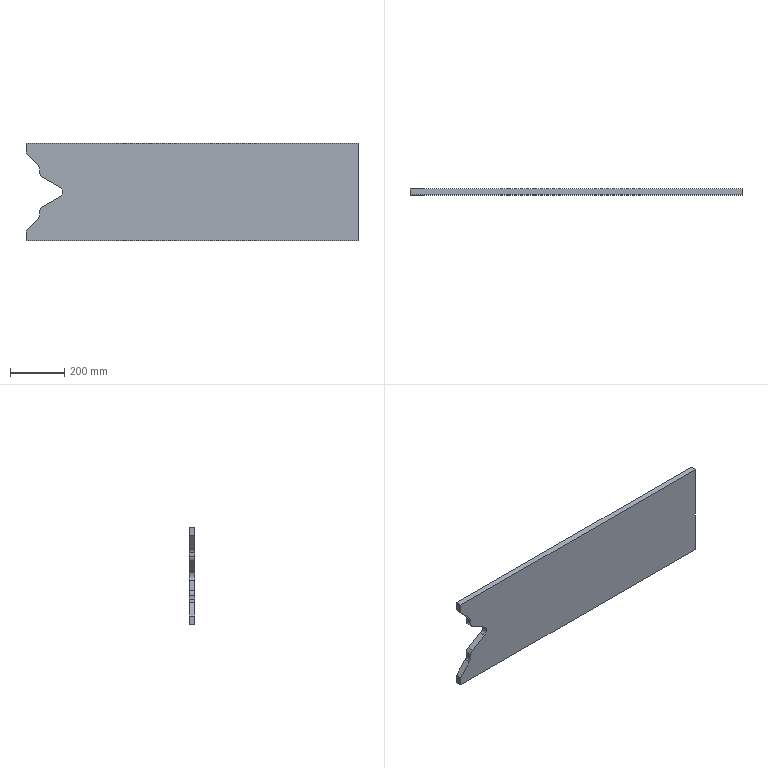Part | NX | features 底座(默认<按焊接>) 2 | 1 solid | 18 faces | box 1222 x 21.82 x 360 mm | volume 9202426 mm3 | plane 13 | cylinder 5 | commonest cylinder face diameters 40 x4 42 x1
STEP:
#1=CARTESIAN_POINT('',(2311.685,545.5,-58.7));
#2=VERTEX_POINT('',#1);
#3=CARTESIAN_POINT('',(2311.685,567.32,-58.7));
#4=VERTEX_POINT('',#3);
#5=CARTESIAN_POINT('',(2311.685,567.32,-58.7));
#6=DIRECTION('',(0.,1.,0.));
#7=VECTOR('',#6,1000.);
#8=LINE('',#5,#7);
#9=EDGE_CURVE('',#2,#4,#8,.T.);
#10=ORIENTED_EDGE('',*,*,#9,.F.);
#11=CARTESIAN_POINT('',(2311.685,545.5,-26.));
#12=VERTEX_POINT('',#11);
#13=CARTESIAN_POINT('',(2311.685,545.5,-386.));
#14=DIRECTION('',(0.,0.,1.));
#15=VECTOR('',#14,1000.);
#16=LINE('',#13,#15);
#17=EDGE_CURVE('',#2,#12,#16,.T.);
#18=ORIENTED_EDGE('',*,*,#17,.T.);
#19=CARTESIAN_POINT('',(2311.685,567.32,-26.));
#20=VERTEX_POINT('',#19);
#21=CARTESIAN_POINT('',(2311.685,567.32,-26.));
#22=DIRECTION('',(0.,-1.,0.));
#23=VECTOR('',#22,1000.);
#24=LINE('',#21,#23);
#25=EDGE_CURVE('',#20,#12,#24,.T.);
#26=ORIENTED_EDGE('',*,*,#25,.F.);
#27=CARTESIAN_POINT('',(2311.685,567.32,-386.));
#28=DIRECTION('',(0.,0.,1.));
#29=VECTOR('',#28,1000.);
#30=LINE('',#27,#29);
#31=EDGE_CURVE('',#4,#20,#30,.T.);
#32=ORIENTED_EDGE('',*,*,#31,.F.);
#33=EDGE_LOOP('',(#10,#18,#26,#32));
#34=FACE_BOUND('',#33,.T.);
#35=CARTESIAN_POINT('',(2311.685,567.32,-386.));
#36=DIRECTION('',(-1.,0.,0.));
#37=DIRECTION('',(0.,0.,1.));
#38=AXIS2_PLACEMENT_3D('',#35,#36,#37);
#39=PLANE('',#38);
#40=ADVANCED_FACE('',(#34),#39,.T.);
#41=CARTESIAN_POINT('',(3533.685,567.32,-26.));
#42=VERTEX_POINT('',#41);
#43=CARTESIAN_POINT('',(3533.685,545.5,-26.));
#44=VERTEX_POINT('',#43);
#45=CARTESIAN_POINT('',(3533.685,567.32,-26.));
#46=DIRECTION('',(0.,-1.,0.));
#47=VECTOR('',#46,1000.);
#48=LINE('',#45,#47);
#49=EDGE_CURVE('',#42,#44,#48,.T.);
#50=ORIENTED_EDGE('',*,*,#49,.F.);
#51=CARTESIAN_POINT('',(3533.685,567.32,-26.));
#52=DIRECTION('',(-1.,0.,0.));
#53=VECTOR('',#52,1000.);
#54=LINE('',#51,#53);
#55=EDGE_CURVE('',#42,#20,#54,.T.);
#56=ORIENTED_EDGE('',*,*,#55,.T.);
#57=ORIENTED_EDGE('',*,*,#25,.T.);
#58=CARTESIAN_POINT('',(3533.685,545.5,-26.));
#59=DIRECTION('',(-1.,0.,0.));
#60=VECTOR('',#59,1000.);
#61=LINE('',#58,#60);
#62=EDGE_CURVE('',#44,#12,#61,.T.);
#63=ORIENTED_EDGE('',*,*,#62,.F.);
#64=EDGE_LOOP('',(#50,#56,#57,#63));
#65=FACE_BOUND('',#64,.T.);
#66=CARTESIAN_POINT('',(3533.685,545.5,-26.));
#67=DIRECTION('',(0.,0.,-1.));
#68=DIRECTION('',(-1.,0.,0.));
#69=AXIS2_PLACEMENT_3D('',#66,#67,#68);
#70=PLANE('',#69);
#71=ADVANCED_FACE('',(#65),#70,.F.);
#72=CARTESIAN_POINT('',(3533.685,567.32,-386.));
#73=VERTEX_POINT('',#72);
#74=CARTESIAN_POINT('',(3533.685,545.5,-386.));
#75=VERTEX_POINT('',#74);
#76=CARTESIAN_POINT('',(3533.685,567.32,-386.));
#77=DIRECTION('',(0.,-1.,0.));
#78=VECTOR('',#77,1000.);
#79=LINE('',#76,#78);
#80=EDGE_CURVE('',#73,#75,#79,.T.);
#81=ORIENTED_EDGE('',*,*,#80,.T.);
#82=CARTESIAN_POINT('',(2311.685,545.5,-386.));
#83=VERTEX_POINT('',#82);
#84=CARTESIAN_POINT('',(3533.685,545.5,-386.));
#85=DIRECTION('',(-1.,0.,0.));
#86=VECTOR('',#85,1000.);
#87=LINE('',#84,#86);
#88=EDGE_CURVE('',#75,#83,#87,.T.);
#89=ORIENTED_EDGE('',*,*,#88,.T.);
#90=CARTESIAN_POINT('',(2311.685,567.32,-386.));
#91=VERTEX_POINT('',#90);
#92=CARTESIAN_POINT('',(2311.685,567.32,-386.));
#93=DIRECTION('',(0.,-1.,0.));
#94=VECTOR('',#93,1000.);
#95=LINE('',#92,#94);
#96=EDGE_CURVE('',#91,#83,#95,.T.);
#97=ORIENTED_EDGE('',*,*,#96,.F.);
#98=CARTESIAN_POINT('',(3533.685,567.32,-386.));
#99=DIRECTION('',(-1.,0.,0.));
#100=VECTOR('',#99,1000.);
#101=LINE('',#98,#100);
#102=EDGE_CURVE('',#73,#91,#101,.T.);
#103=ORIENTED_EDGE('',*,*,#102,.F.);
#104=EDGE_LOOP('',(#81,#89,#97,#103));
#105=FACE_BOUND('',#104,.T.);
#106=CARTESIAN_POINT('',(3533.685,545.5,-386.));
#107=DIRECTION('',(0.,0.,-1.));
#108=DIRECTION('',(-1.,0.,0.));
#109=AXIS2_PLACEMENT_3D('',#106,#107,#108);
#110=PLANE('',#109);
#111=ADVANCED_FACE('',(#105),#110,.T.);
#112=CARTESIAN_POINT('',(2311.685,567.32,-353.3));
#113=VERTEX_POINT('',#112);
#114=CARTESIAN_POINT('',(2311.685,545.5,-353.3));
#115=VERTEX_POINT('',#114);
#116=CARTESIAN_POINT('',(2311.685,567.32,-353.3));
#117=DIRECTION('',(0.,-1.,0.));
#118=VECTOR('',#117,1000.);
#119=LINE('',#116,#118);
#120=EDGE_CURVE('',#113,#115,#119,.T.);
#121=ORIENTED_EDGE('',*,*,#120,.F.);
#122=CARTESIAN_POINT('',(2311.685,567.32,-386.));
#123=DIRECTION('',(0.,0.,1.));
#124=VECTOR('',#123,1000.);
#125=LINE('',#122,#124);
#126=EDGE_CURVE('',#91,#113,#125,.T.);
#127=ORIENTED_EDGE('',*,*,#126,.F.);
#128=ORIENTED_EDGE('',*,*,#96,.T.);
#129=CARTESIAN_POINT('',(2311.685,545.5,-386.));
#130=DIRECTION('',(0.,0.,1.));
#131=VECTOR('',#130,1000.);
#132=LINE('',#129,#131);
#133=EDGE_CURVE('',#83,#115,#132,.T.);
#134=ORIENTED_EDGE('',*,*,#133,.T.);
#135=EDGE_LOOP('',(#121,#127,#128,#134));
#136=FACE_BOUND('',#135,.T.);
#137=CARTESIAN_POINT('',(2311.685,567.32,-386.));
#138=DIRECTION('',(-1.,0.,0.));
#139=DIRECTION('',(0.,0.,1.));
#140=AXIS2_PLACEMENT_3D('',#137,#138,#139);
#141=PLANE('',#140);
#142=ADVANCED_FACE('',(#136),#141,.T.);
#143=ORIENTED_EDGE('',*,*,#17,.F.);
#144=CARTESIAN_POINT('',(2356.433,545.5,-107.546));
#145=VERTEX_POINT('',#144);
#146=CARTESIAN_POINT('',(2311.685,545.5,-58.7));
#147=DIRECTION('',(-0.6755,0.,0.7374));
#148=VECTOR('',#147,1000.);
#149=LINE('',#146,#148);
#150=EDGE_CURVE('',#145,#2,#149,.T.);
#151=ORIENTED_EDGE('',*,*,#150,.F.);
#152=CARTESIAN_POINT('',(2361.685,545.5,-121.056));
#153=VERTEX_POINT('',#152);
#154=CARTESIAN_POINT('',(2341.685,545.5,-121.056));
#155=DIRECTION('',(0.,-1.,0.));
#156=DIRECTION('',(0.,0.,-1.));
#157=AXIS2_PLACEMENT_3D('',#154,#155,#156);
#158=CIRCLE('',#157,20.);
#159=EDGE_CURVE('',#153,#145,#158,.T.);
#160=ORIENTED_EDGE('',*,*,#159,.F.);
#161=CARTESIAN_POINT('',(2361.685,545.5,-133.717));
#162=VERTEX_POINT('',#161);
#163=CARTESIAN_POINT('',(2361.685,545.5,-121.056));
#164=DIRECTION('',(0.,0.,1.));
#165=VECTOR('',#164,1000.);
#166=LINE('',#163,#165);
#167=EDGE_CURVE('',#162,#153,#166,.T.);
#168=ORIENTED_EDGE('',*,*,#167,.F.);
#169=CARTESIAN_POINT('',(2372.64,545.5,-151.555));
#170=VERTEX_POINT('',#169);
#171=CARTESIAN_POINT('',(2381.685,545.5,-133.717));
#172=DIRECTION('',(0.,1.,0.));
#173=DIRECTION('',(0.,0.,1.));
#174=AXIS2_PLACEMENT_3D('',#171,#172,#173);
#175=CIRCLE('',#174,20.);
#176=EDGE_CURVE('',#170,#162,#175,.T.);
#177=ORIENTED_EDGE('',*,*,#176,.F.);
#178=CARTESIAN_POINT('',(2436.093,545.5,-187.76));
#179=VERTEX_POINT('',#178);
#180=CARTESIAN_POINT('',(2372.64,545.5,-151.555));
#181=DIRECTION('',(-0.8686,0.,0.4956));
#182=VECTOR('',#181,1000.);
#183=LINE('',#180,#182);
#184=EDGE_CURVE('',#179,#170,#183,.T.);
#185=ORIENTED_EDGE('',*,*,#184,.F.);
#186=CARTESIAN_POINT('',(2436.093,545.5,-224.24));
#187=VERTEX_POINT('',#186);
#188=CARTESIAN_POINT('',(2425.685,545.5,-206.));
#189=DIRECTION('',(0.,-1.,0.));
#190=DIRECTION('',(0.,0.,-1.));
#191=AXIS2_PLACEMENT_3D('',#188,#189,#190);
#192=CIRCLE('',#191,21.);
#193=EDGE_CURVE('',#187,#179,#192,.T.);
#194=ORIENTED_EDGE('',*,*,#193,.F.);
#195=CARTESIAN_POINT('',(2372.64,545.5,-260.445));
#196=VERTEX_POINT('',#195);
#197=CARTESIAN_POINT('',(2372.64,545.5,-260.445));
#198=DIRECTION('',(0.8686,0.,0.4956));
#199=VECTOR('',#198,1000.);
#200=LINE('',#197,#199);
#201=EDGE_CURVE('',#196,#187,#200,.T.);
#202=ORIENTED_EDGE('',*,*,#201,.F.);
#203=CARTESIAN_POINT('',(2361.685,545.5,-278.283));
#204=VERTEX_POINT('',#203);
#205=CARTESIAN_POINT('',(2381.685,545.5,-278.283));
#206=DIRECTION('',(0.,1.,0.));
#207=DIRECTION('',(0.,0.,-1.));
#208=AXIS2_PLACEMENT_3D('',#205,#206,#207);
#209=CIRCLE('',#208,20.);
#210=EDGE_CURVE('',#204,#196,#209,.T.);
#211=ORIENTED_EDGE('',*,*,#210,.F.);
#212=CARTESIAN_POINT('',(2361.685,545.5,-290.944));
#213=VERTEX_POINT('',#212);
#214=CARTESIAN_POINT('',(2361.685,545.5,-290.944));
#215=DIRECTION('',(0.,0.,1.));
#216=VECTOR('',#215,1000.);
#217=LINE('',#214,#216);
#218=EDGE_CURVE('',#213,#204,#217,.T.);
#219=ORIENTED_EDGE('',*,*,#218,.F.);
#220=CARTESIAN_POINT('',(2356.433,545.5,-304.454));
#221=VERTEX_POINT('',#220);
#222=CARTESIAN_POINT('',(2341.685,545.5,-290.944));
#223=DIRECTION('',(0.,-1.,0.));
#224=DIRECTION('',(0.,0.,1.));
#225=AXIS2_PLACEMENT_3D('',#222,#223,#224);
#226=CIRCLE('',#225,20.);
#227=EDGE_CURVE('',#221,#213,#226,.T.);
#228=ORIENTED_EDGE('',*,*,#227,.F.);
#229=CARTESIAN_POINT('',(2311.685,545.5,-353.3));
#230=DIRECTION('',(0.6755,0.,0.7374));
#231=VECTOR('',#230,1000.);
#232=LINE('',#229,#231);
#233=EDGE_CURVE('',#115,#221,#232,.T.);
#234=ORIENTED_EDGE('',*,*,#233,.F.);
#235=ORIENTED_EDGE('',*,*,#133,.F.);
#236=ORIENTED_EDGE('',*,*,#88,.F.);
#237=CARTESIAN_POINT('',(3533.685,545.5,-386.));
#238=DIRECTION('',(0.,0.,1.));
#239=VECTOR('',#238,1000.);
#240=LINE('',#237,#239);
#241=EDGE_CURVE('',#75,#44,#240,.T.);
#242=ORIENTED_EDGE('',*,*,#241,.T.);
#243=ORIENTED_EDGE('',*,*,#62,.T.);
#244=EDGE_LOOP('',(#143,#151,#160,#168,#177,#185,#194,#202,#211,#219,#228,#234,#235,#236,#242,#243));
#245=FACE_BOUND('',#244,.T.);
#246=CARTESIAN_POINT('',(3533.685,545.5,-386.));
#247=DIRECTION('',(0.,1.,0.));
#248=DIRECTION('',(0.,0.,1.));
#249=AXIS2_PLACEMENT_3D('',#246,#247,#248);
#250=PLANE('',#249);
#251=ADVANCED_FACE('',(#245),#250,.F.);
#252=ORIENTED_EDGE('',*,*,#49,.T.);
#253=ORIENTED_EDGE('',*,*,#241,.F.);
#254=ORIENTED_EDGE('',*,*,#80,.F.);
#255=CARTESIAN_POINT('',(3533.685,567.32,-386.));
#256=DIRECTION('',(0.,0.,1.));
#257=VECTOR('',#256,1000.);
#258=LINE('',#255,#257);
#259=EDGE_CURVE('',#73,#42,#258,.T.);
#260=ORIENTED_EDGE('',*,*,#259,.T.);
#261=EDGE_LOOP('',(#252,#253,#254,#260));
#262=FACE_BOUND('',#261,.T.);
#263=CARTESIAN_POINT('',(3533.685,567.32,-386.));
#264=DIRECTION('',(-1.,0.,0.));
#265=DIRECTION('',(0.,0.,1.));
#266=AXIS2_PLACEMENT_3D('',#263,#264,#265);
#267=PLANE('',#266);
#268=ADVANCED_FACE('',(#262),#267,.F.);
#269=CARTESIAN_POINT('',(2356.433,567.32,-107.546));
#270=VERTEX_POINT('',#269);
#271=CARTESIAN_POINT('',(3032.295,567.32,-845.317));
#272=DIRECTION('',(0.6755,0.,-0.7374));
#273=VECTOR('',#272,1000.);
#274=LINE('',#271,#273);
#275=EDGE_CURVE('',#4,#270,#274,.T.);
#276=ORIENTED_EDGE('',*,*,#275,.F.);
#277=ORIENTED_EDGE('',*,*,#31,.T.);
#278=ORIENTED_EDGE('',*,*,#55,.F.);
#279=ORIENTED_EDGE('',*,*,#259,.F.);
#280=ORIENTED_EDGE('',*,*,#102,.T.);
#281=ORIENTED_EDGE('',*,*,#126,.T.);
#282=CARTESIAN_POINT('',(2356.433,567.32,-304.454));
#283=VERTEX_POINT('',#282);
#284=CARTESIAN_POINT('',(2852.984,567.32,237.581));
#285=DIRECTION('',(-0.6755,0.,-0.7374));
#286=VECTOR('',#285,1000.);
#287=LINE('',#284,#286);
#288=EDGE_CURVE('',#283,#113,#287,.T.);
#289=ORIENTED_EDGE('',*,*,#288,.F.);
#290=CARTESIAN_POINT('',(2361.685,567.32,-290.944));
#291=VERTEX_POINT('',#290);
#292=CARTESIAN_POINT('',(2341.685,567.32,-290.944));
#293=DIRECTION('',(0.,1.,0.));
#294=DIRECTION('',(0.,0.,1.));
#295=AXIS2_PLACEMENT_3D('',#292,#293,#294);
#296=CIRCLE('',#295,20.);
#297=EDGE_CURVE('',#291,#283,#296,.T.);
#298=ORIENTED_EDGE('',*,*,#297,.F.);
#299=CARTESIAN_POINT('',(2361.685,567.32,-278.283));
#300=VERTEX_POINT('',#299);
#301=CARTESIAN_POINT('',(2361.685,567.32,-386.));
#302=DIRECTION('',(0.,0.,-1.));
#303=VECTOR('',#302,1000.);
#304=LINE('',#301,#303);
#305=EDGE_CURVE('',#300,#291,#304,.T.);
#306=ORIENTED_EDGE('',*,*,#305,.F.);
#307=CARTESIAN_POINT('',(2372.64,567.32,-260.445));
#308=VERTEX_POINT('',#307);
#309=CARTESIAN_POINT('',(2381.685,567.32,-278.283));
#310=DIRECTION('',(0.,1.,0.));
#311=DIRECTION('',(0.,0.,1.));
#312=AXIS2_PLACEMENT_3D('',#309,#310,#311);
#313=CIRCLE('',#312,20.);
#314=EDGE_CURVE('',#308,#300,#313,.F.);
#315=ORIENTED_EDGE('',*,*,#314,.F.);
#316=CARTESIAN_POINT('',(2436.093,567.32,-224.24));
#317=VERTEX_POINT('',#316);
#318=CARTESIAN_POINT('',(3194.48,567.32,208.486));
#319=DIRECTION('',(-0.8686,0.,-0.4956));
#320=VECTOR('',#319,1000.);
#321=LINE('',#318,#320);
#322=EDGE_CURVE('',#317,#308,#321,.T.);
#323=ORIENTED_EDGE('',*,*,#322,.F.);
#324=CARTESIAN_POINT('',(2436.093,567.32,-187.76));
#325=VERTEX_POINT('',#324);
#326=CARTESIAN_POINT('',(2425.685,567.32,-206.));
#327=DIRECTION('',(0.,1.,0.));
#328=DIRECTION('',(0.,0.,1.));
#329=AXIS2_PLACEMENT_3D('',#326,#327,#328);
#330=CIRCLE('',#329,21.);
#331=EDGE_CURVE('',#325,#317,#330,.T.);
#332=ORIENTED_EDGE('',*,*,#331,.F.);
#333=CARTESIAN_POINT('',(2372.64,567.32,-151.555));
#334=VERTEX_POINT('',#333);
#335=CARTESIAN_POINT('',(3349.441,567.32,-708.904));
#336=DIRECTION('',(0.8686,0.,-0.4956));
#337=VECTOR('',#336,1000.);
#338=LINE('',#335,#337);
#339=EDGE_CURVE('',#334,#325,#338,.T.);
#340=ORIENTED_EDGE('',*,*,#339,.F.);
#341=CARTESIAN_POINT('',(2361.685,567.32,-133.717));
#342=VERTEX_POINT('',#341);
#343=CARTESIAN_POINT('',(2381.685,567.32,-133.717));
#344=DIRECTION('',(0.,1.,0.));
#345=DIRECTION('',(0.,0.,1.));
#346=AXIS2_PLACEMENT_3D('',#343,#344,#345);
#347=CIRCLE('',#346,20.);
#348=EDGE_CURVE('',#342,#334,#347,.F.);
#349=ORIENTED_EDGE('',*,*,#348,.F.);
#350=CARTESIAN_POINT('',(2361.685,567.32,-121.056));
#351=VERTEX_POINT('',#350);
#352=CARTESIAN_POINT('',(2361.685,567.32,-386.));
#353=DIRECTION('',(0.,0.,-1.));
#354=VECTOR('',#353,1000.);
#355=LINE('',#352,#354);
#356=EDGE_CURVE('',#351,#342,#355,.T.);
#357=ORIENTED_EDGE('',*,*,#356,.F.);
#358=CARTESIAN_POINT('',(2341.685,567.32,-121.056));
#359=DIRECTION('',(0.,1.,0.));
#360=DIRECTION('',(0.,0.,1.));
#361=AXIS2_PLACEMENT_3D('',#358,#359,#360);
#362=CIRCLE('',#361,20.);
#363=EDGE_CURVE('',#270,#351,#362,.T.);
#364=ORIENTED_EDGE('',*,*,#363,.F.);
#365=EDGE_LOOP('',(#276,#277,#278,#279,#280,#281,#289,#298,#306,#315,#323,#332,#340,#349,#357,#364));
#366=FACE_BOUND('',#365,.T.);
#367=CARTESIAN_POINT('',(3533.685,567.32,-386.));
#368=DIRECTION('',(0.,1.,0.));
#369=DIRECTION('',(0.,0.,1.));
#370=AXIS2_PLACEMENT_3D('',#367,#368,#369);
#371=PLANE('',#370);
#372=ADVANCED_FACE('',(#366),#371,.T.);
#373=ORIENTED_EDGE('',*,*,#275,.T.);
#374=CARTESIAN_POINT('',(2356.433,584.776,-107.546));
#375=DIRECTION('',(0.,-1.,0.));
#376=VECTOR('',#375,1000.);
#377=LINE('',#374,#376);
#378=EDGE_CURVE('',#270,#145,#377,.T.);
#379=ORIENTED_EDGE('',*,*,#378,.T.);
#380=ORIENTED_EDGE('',*,*,#150,.T.);
#381=ORIENTED_EDGE('',*,*,#9,.T.);
#382=EDGE_LOOP('',(#373,#379,#380,#381));
#383=FACE_BOUND('',#382,.T.);
#384=CARTESIAN_POINT('',(2311.685,584.776,-58.7));
#385=DIRECTION('',(0.7374,0.,0.6755));
#386=DIRECTION('',(0.6755,0.,-0.7374));
#387=AXIS2_PLACEMENT_3D('',#384,#385,#386);
#388=PLANE('',#387);
#389=ADVANCED_FACE('',(#383),#388,.F.);
#390=ORIENTED_EDGE('',*,*,#363,.T.);
#391=CARTESIAN_POINT('',(2361.685,584.776,-121.056));
#392=DIRECTION('',(0.,-1.,0.));
#393=VECTOR('',#392,1000.);
#394=LINE('',#391,#393);
#395=EDGE_CURVE('',#351,#153,#394,.T.);
#396=ORIENTED_EDGE('',*,*,#395,.T.);
#397=ORIENTED_EDGE('',*,*,#159,.T.);
#398=ORIENTED_EDGE('',*,*,#378,.F.);
#399=EDGE_LOOP('',(#390,#396,#397,#398));
#400=FACE_BOUND('',#399,.T.);
#401=CARTESIAN_POINT('',(2341.685,584.776,-121.056));
#402=DIRECTION('',(0.,-1.,0.));
#403=DIRECTION('',(0.,0.,-1.));
#404=AXIS2_PLACEMENT_3D('',#401,#402,#403);
#405=CYLINDRICAL_SURFACE('',#404,20.);
#406=ADVANCED_FACE('',(#400),#405,.F.);
#407=ORIENTED_EDGE('',*,*,#356,.T.);
#408=CARTESIAN_POINT('',(2361.685,584.776,-133.717));
#409=DIRECTION('',(0.,-1.,0.));
#410=VECTOR('',#409,1000.);
#411=LINE('',#408,#410);
#412=EDGE_CURVE('',#342,#162,#411,.T.);
#413=ORIENTED_EDGE('',*,*,#412,.T.);
#414=ORIENTED_EDGE('',*,*,#167,.T.);
#415=ORIENTED_EDGE('',*,*,#395,.F.);
#416=EDGE_LOOP('',(#407,#413,#414,#415));
#417=FACE_BOUND('',#416,.T.);
#418=CARTESIAN_POINT('',(2361.685,584.776,-121.056));
#419=DIRECTION('',(1.,0.,0.));
#420=DIRECTION('',(0.,0.,-1.));
#421=AXIS2_PLACEMENT_3D('',#418,#419,#420);
#422=PLANE('',#421);
#423=ADVANCED_FACE('',(#417),#422,.F.);
#424=ORIENTED_EDGE('',*,*,#348,.T.);
#425=CARTESIAN_POINT('',(2372.64,584.776,-151.555));
#426=DIRECTION('',(0.,-1.,0.));
#427=VECTOR('',#426,1000.);
#428=LINE('',#425,#427);
#429=EDGE_CURVE('',#334,#170,#428,.T.);
#430=ORIENTED_EDGE('',*,*,#429,.T.);
#431=ORIENTED_EDGE('',*,*,#176,.T.);
#432=ORIENTED_EDGE('',*,*,#412,.F.);
#433=EDGE_LOOP('',(#424,#430,#431,#432));
#434=FACE_BOUND('',#433,.T.);
#435=CARTESIAN_POINT('',(2381.685,584.776,-133.717));
#436=DIRECTION('',(0.,-1.,0.));
#437=DIRECTION('',(0.,0.,-1.));
#438=AXIS2_PLACEMENT_3D('',#435,#436,#437);
#439=CYLINDRICAL_SURFACE('',#438,20.);
#440=ADVANCED_FACE('',(#434),#439,.T.);
#441=ORIENTED_EDGE('',*,*,#339,.T.);
#442=CARTESIAN_POINT('',(2436.093,584.776,-187.76));
#443=DIRECTION('',(0.,-1.,0.));
#444=VECTOR('',#443,1000.);
#445=LINE('',#442,#444);
#446=EDGE_CURVE('',#325,#179,#445,.T.);
#447=ORIENTED_EDGE('',*,*,#446,.T.);
#448=ORIENTED_EDGE('',*,*,#184,.T.);
#449=ORIENTED_EDGE('',*,*,#429,.F.);
#450=EDGE_LOOP('',(#441,#447,#448,#449));
#451=FACE_BOUND('',#450,.T.);
#452=CARTESIAN_POINT('',(2372.64,584.776,-151.555));
#453=DIRECTION('',(0.4956,0.,0.8686));
#454=DIRECTION('',(0.8686,0.,-0.4956));
#455=AXIS2_PLACEMENT_3D('',#452,#453,#454);
#456=PLANE('',#455);
#457=ADVANCED_FACE('',(#451),#456,.F.);
#458=ORIENTED_EDGE('',*,*,#331,.T.);
#459=CARTESIAN_POINT('',(2436.093,584.776,-224.24));
#460=DIRECTION('',(0.,-1.,0.));
#461=VECTOR('',#460,1000.);
#462=LINE('',#459,#461);
#463=EDGE_CURVE('',#317,#187,#462,.T.);
#464=ORIENTED_EDGE('',*,*,#463,.T.);
#465=ORIENTED_EDGE('',*,*,#193,.T.);
#466=ORIENTED_EDGE('',*,*,#446,.F.);
#467=EDGE_LOOP('',(#458,#464,#465,#466));
#468=FACE_BOUND('',#467,.T.);
#469=CARTESIAN_POINT('',(2425.685,584.776,-206.));
#470=DIRECTION('',(0.,-1.,0.));
#471=DIRECTION('',(0.,0.,-1.));
#472=AXIS2_PLACEMENT_3D('',#469,#470,#471);
#473=CYLINDRICAL_SURFACE('',#472,21.);
#474=ADVANCED_FACE('',(#468),#473,.F.);
#475=ORIENTED_EDGE('',*,*,#322,.T.);
#476=CARTESIAN_POINT('',(2372.64,584.776,-260.445));
#477=DIRECTION('',(0.,-1.,0.));
#478=VECTOR('',#477,1000.);
#479=LINE('',#476,#478);
#480=EDGE_CURVE('',#308,#196,#479,.T.);
#481=ORIENTED_EDGE('',*,*,#480,.T.);
#482=ORIENTED_EDGE('',*,*,#201,.T.);
#483=ORIENTED_EDGE('',*,*,#463,.F.);
#484=EDGE_LOOP('',(#475,#481,#482,#483));
#485=FACE_BOUND('',#484,.T.);
#486=CARTESIAN_POINT('',(2372.64,584.776,-260.445));
#487=DIRECTION('',(0.4956,0.,-0.8686));
#488=DIRECTION('',(-0.8686,0.,-0.4956));
#489=AXIS2_PLACEMENT_3D('',#486,#487,#488);
#490=PLANE('',#489);
#491=ADVANCED_FACE('',(#485),#490,.F.);
#492=ORIENTED_EDGE('',*,*,#314,.T.);
#493=CARTESIAN_POINT('',(2361.685,584.776,-278.283));
#494=DIRECTION('',(0.,-1.,0.));
#495=VECTOR('',#494,1000.);
#496=LINE('',#493,#495);
#497=EDGE_CURVE('',#300,#204,#496,.T.);
#498=ORIENTED_EDGE('',*,*,#497,.T.);
#499=ORIENTED_EDGE('',*,*,#210,.T.);
#500=ORIENTED_EDGE('',*,*,#480,.F.);
#501=EDGE_LOOP('',(#492,#498,#499,#500));
#502=FACE_BOUND('',#501,.T.);
#503=CARTESIAN_POINT('',(2381.685,584.776,-278.283));
#504=DIRECTION('',(0.,-1.,0.));
#505=DIRECTION('',(0.,0.,-1.));
#506=AXIS2_PLACEMENT_3D('',#503,#504,#505);
#507=CYLINDRICAL_SURFACE('',#506,20.);
#508=ADVANCED_FACE('',(#502),#507,.T.);
#509=ORIENTED_EDGE('',*,*,#305,.T.);
#510=CARTESIAN_POINT('',(2361.685,584.776,-290.944));
#511=DIRECTION('',(0.,-1.,0.));
#512=VECTOR('',#511,1000.);
#513=LINE('',#510,#512);
#514=EDGE_CURVE('',#291,#213,#513,.T.);
#515=ORIENTED_EDGE('',*,*,#514,.T.);
#516=ORIENTED_EDGE('',*,*,#218,.T.);
#517=ORIENTED_EDGE('',*,*,#497,.F.);
#518=EDGE_LOOP('',(#509,#515,#516,#517));
#519=FACE_BOUND('',#518,.T.);
#520=CARTESIAN_POINT('',(2361.685,584.776,-290.944));
#521=DIRECTION('',(1.,0.,0.));
#522=DIRECTION('',(0.,0.,-1.));
#523=AXIS2_PLACEMENT_3D('',#520,#521,#522);
#524=PLANE('',#523);
#525=ADVANCED_FACE('',(#519),#524,.F.);
#526=ORIENTED_EDGE('',*,*,#297,.T.);
#527=CARTESIAN_POINT('',(2356.433,584.776,-304.454));
#528=DIRECTION('',(0.,-1.,0.));
#529=VECTOR('',#528,1000.);
#530=LINE('',#527,#529);
#531=EDGE_CURVE('',#283,#221,#530,.T.);
#532=ORIENTED_EDGE('',*,*,#531,.T.);
#533=ORIENTED_EDGE('',*,*,#227,.T.);
#534=ORIENTED_EDGE('',*,*,#514,.F.);
#535=EDGE_LOOP('',(#526,#532,#533,#534));
#536=FACE_BOUND('',#535,.T.);
#537=CARTESIAN_POINT('',(2341.685,584.776,-290.944));
#538=DIRECTION('',(0.,-1.,0.));
#539=DIRECTION('',(0.,0.,-1.));
#540=AXIS2_PLACEMENT_3D('',#537,#538,#539);
#541=CYLINDRICAL_SURFACE('',#540,20.);
#542=ADVANCED_FACE('',(#536),#541,.F.);
#543=ORIENTED_EDGE('',*,*,#288,.T.);
#544=ORIENTED_EDGE('',*,*,#120,.T.);
#545=ORIENTED_EDGE('',*,*,#233,.T.);
#546=ORIENTED_EDGE('',*,*,#531,.F.);
#547=EDGE_LOOP('',(#543,#544,#545,#546));
#548=FACE_BOUND('',#547,.T.);
#549=CARTESIAN_POINT('',(2311.685,584.776,-353.3));
#550=DIRECTION('',(0.7374,0.,-0.6755));
#551=DIRECTION('',(-0.6755,0.,-0.7374));
#552=AXIS2_PLACEMENT_3D('',#549,#550,#551);
#553=PLANE('',#552);
#554=ADVANCED_FACE('',(#548),#553,.F.);
#555=CLOSED_SHELL('',(#40,#71,#111,#142,#251,#268,#372,#389,#406,#423,#440,#457,#474,#491,#508,#525,#542,#554));
#556=MANIFOLD_SOLID_BREP('',#555);
#557=(LENGTH_UNIT()NAMED_UNIT(*)SI_UNIT(.MILLI.,.METRE.));
#558=UNCERTAINTY_MEASURE_WITH_UNIT(LENGTH_MEASURE(0.00001),#557,'','');
#559=(NAMED_UNIT(*)PLANE_ANGLE_UNIT()SI_UNIT($,.RADIAN.));
#560=(NAMED_UNIT(*)SI_UNIT($,.STERADIAN.)SOLID_ANGLE_UNIT());
#561=(GEOMETRIC_REPRESENTATION_CONTEXT(3)GLOBAL_UNCERTAINTY_ASSIGNED_CONTEXT((#558))GLOBAL_UNIT_ASSIGNED_CONTEXT((#557,#559,#560))REPRESENTATION_CONTEXT('',''));
#562=ADVANCED_BREP_SHAPE_REPRESENTATION('',(#556),#561);